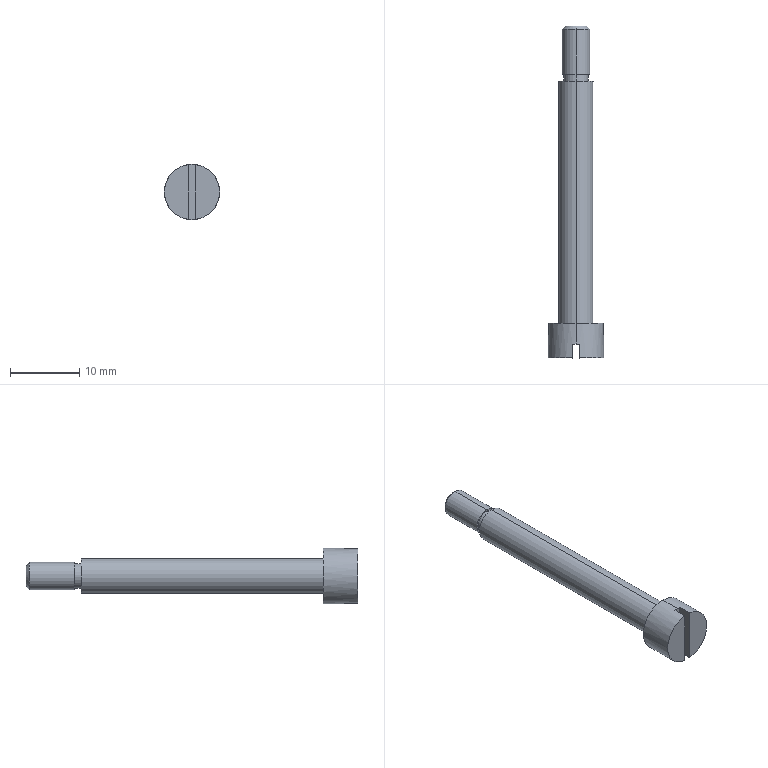Part | STEP file | 03-21 guide screw | 1 solid | 19 faces | box 8 x 48 x 8 mm | volume 1019 mm3 | plane 9 | cylinder 8 | cone 2 | commonest cylinder face diameters 3.5 x2 4 x2 5 x2 8 x2
STEP:
#1=CARTESIAN_POINT('',(0.,7.,1.5));
#2=VERTEX_POINT('',#1);
#3=CARTESIAN_POINT('',(0.,7.,-1.5));
#4=VERTEX_POINT('',#3);
#5=CARTESIAN_POINT('',(0.,7.,0.));
#6=DIRECTION('',(0.,1.,0.));
#7=DIRECTION('',(0.,0.,1.));
#8=AXIS2_PLACEMENT_3D('',#5,#6,#7);
#9=CIRCLE('',#8,1.5);
#10=EDGE_CURVE('',#2,#4,#9,.T.);
#11=ORIENTED_EDGE('',*,*,#10,.F.);
#12=CARTESIAN_POINT('',(0.,6.5,2.));
#13=VERTEX_POINT('',#12);
#14=CARTESIAN_POINT('',(0.,7.,1.5));
#15=DIRECTION('',(0.,-0.7071,0.7071));
#16=VECTOR('',#15,1000.);
#17=LINE('',#14,#16);
#18=EDGE_CURVE('',#2,#13,#17,.T.);
#19=ORIENTED_EDGE('',*,*,#18,.T.);
#20=CARTESIAN_POINT('',(0.,6.5,-2.));
#21=VERTEX_POINT('',#20);
#22=CARTESIAN_POINT('',(0.,6.5,0.));
#23=DIRECTION('',(0.,-1.,0.));
#24=DIRECTION('',(0.,0.,1.));
#25=AXIS2_PLACEMENT_3D('',#22,#23,#24);
#26=CIRCLE('',#25,2.);
#27=EDGE_CURVE('',#21,#13,#26,.T.);
#28=ORIENTED_EDGE('',*,*,#27,.F.);
#29=CARTESIAN_POINT('',(0.,7.,-1.5));
#30=DIRECTION('',(0.,-0.7071,-0.7071));
#31=VECTOR('',#30,1000.);
#32=LINE('',#29,#31);
#33=EDGE_CURVE('',#4,#21,#32,.T.);
#34=ORIENTED_EDGE('',*,*,#33,.F.);
#35=EDGE_LOOP('',(#11,#19,#28,#34));
#36=FACE_OUTER_BOUND('',#35,.T.);
#37=CARTESIAN_POINT('',(0.,7.,0.));
#38=DIRECTION('',(0.,-1.,0.));
#39=DIRECTION('',(0.,0.,-1.));
#40=AXIS2_PLACEMENT_3D('',#37,#38,#39);
#41=CONICAL_SURFACE('',#40,1.5,0.7854);
#42=ADVANCED_FACE('',(#36),#41,.T.);
#43=CARTESIAN_POINT('',(0.,-39.,-4.));
#44=VERTEX_POINT('',#43);
#45=CARTESIAN_POINT('',(0.5,-39.,-3.969));
#46=VERTEX_POINT('',#45);
#47=CARTESIAN_POINT('',(0.,-39.,0.));
#48=DIRECTION('',(0.,-1.,0.));
#49=DIRECTION('',(0.,0.,-1.));
#50=AXIS2_PLACEMENT_3D('',#47,#48,#49);
#51=CIRCLE('',#50,4.);
#52=EDGE_CURVE('',#44,#46,#51,.T.);
#53=ORIENTED_EDGE('',*,*,#52,.F.);
#54=CARTESIAN_POINT('',(0.,-36.,-4.));
#55=VERTEX_POINT('',#54);
#56=CARTESIAN_POINT('',(0.,-41.,-4.));
#57=DIRECTION('',(0.,1.,0.));
#58=VECTOR('',#57,1000.);
#59=LINE('',#56,#58);
#60=EDGE_CURVE('',#44,#55,#59,.T.);
#61=ORIENTED_EDGE('',*,*,#60,.T.);
#62=CARTESIAN_POINT('',(0.,-36.,4.));
#63=VERTEX_POINT('',#62);
#64=CARTESIAN_POINT('',(0.,-36.,0.));
#65=DIRECTION('',(0.,-1.,0.));
#66=DIRECTION('',(0.,0.,-1.));
#67=AXIS2_PLACEMENT_3D('',#64,#65,#66);
#68=CIRCLE('',#67,4.);
#69=EDGE_CURVE('',#55,#63,#68,.T.);
#70=ORIENTED_EDGE('',*,*,#69,.T.);
#71=CARTESIAN_POINT('',(0.,-39.,4.));
#72=VERTEX_POINT('',#71);
#73=CARTESIAN_POINT('',(0.,-41.,4.));
#74=DIRECTION('',(0.,1.,0.));
#75=VECTOR('',#74,1000.);
#76=LINE('',#73,#75);
#77=EDGE_CURVE('',#72,#63,#76,.T.);
#78=ORIENTED_EDGE('',*,*,#77,.F.);
#79=CARTESIAN_POINT('',(0.5,-39.,3.969));
#80=VERTEX_POINT('',#79);
#81=CARTESIAN_POINT('',(0.,-39.,0.));
#82=DIRECTION('',(0.,-1.,0.));
#83=DIRECTION('',(0.,0.,-1.));
#84=AXIS2_PLACEMENT_3D('',#81,#82,#83);
#85=CIRCLE('',#84,4.);
#86=EDGE_CURVE('',#80,#72,#85,.T.);
#87=ORIENTED_EDGE('',*,*,#86,.F.);
#88=CARTESIAN_POINT('',(0.5,-41.,3.969));
#89=VERTEX_POINT('',#88);
#90=CARTESIAN_POINT('',(0.5,-41.,3.969));
#91=DIRECTION('',(0.,-1.,0.));
#92=VECTOR('',#91,1000.);
#93=LINE('',#90,#92);
#94=EDGE_CURVE('',#80,#89,#93,.T.);
#95=ORIENTED_EDGE('',*,*,#94,.T.);
#96=CARTESIAN_POINT('',(0.5,-41.,-3.969));
#97=VERTEX_POINT('',#96);
#98=CARTESIAN_POINT('',(0.,-41.,0.));
#99=DIRECTION('',(0.,-1.,0.));
#100=DIRECTION('',(0.,0.,-1.));
#101=AXIS2_PLACEMENT_3D('',#98,#99,#100);
#102=CIRCLE('',#101,4.);
#103=EDGE_CURVE('',#97,#89,#102,.T.);
#104=ORIENTED_EDGE('',*,*,#103,.F.);
#105=CARTESIAN_POINT('',(0.5,-41.,-3.969));
#106=DIRECTION('',(0.,1.,0.));
#107=VECTOR('',#106,1000.);
#108=LINE('',#105,#107);
#109=EDGE_CURVE('',#97,#46,#108,.T.);
#110=ORIENTED_EDGE('',*,*,#109,.T.);
#111=EDGE_LOOP('',(#53,#61,#70,#78,#87,#95,#104,#110));
#112=FACE_OUTER_BOUND('',#111,.T.);
#113=CARTESIAN_POINT('',(0.,-41.,0.));
#114=DIRECTION('',(0.,1.,0.));
#115=DIRECTION('',(0.,0.,1.));
#116=AXIS2_PLACEMENT_3D('',#113,#114,#115);
#117=CYLINDRICAL_SURFACE('',#116,4.);
#118=ADVANCED_FACE('',(#112),#117,.T.);
#119=CARTESIAN_POINT('',(0.,-36.,-2.5));
#120=VERTEX_POINT('',#119);
#121=CARTESIAN_POINT('',(0.,-36.,2.5));
#122=VERTEX_POINT('',#121);
#123=CARTESIAN_POINT('',(0.,-36.,0.));
#124=DIRECTION('',(0.,-1.,0.));
#125=DIRECTION('',(0.,0.,-1.));
#126=AXIS2_PLACEMENT_3D('',#123,#124,#125);
#127=CIRCLE('',#126,2.5);
#128=EDGE_CURVE('',#120,#122,#127,.T.);
#129=ORIENTED_EDGE('',*,*,#128,.F.);
#130=CARTESIAN_POINT('',(0.,-1.,-2.5));
#131=VERTEX_POINT('',#130);
#132=CARTESIAN_POINT('',(0.,-36.,-2.5));
#133=DIRECTION('',(0.,1.,0.));
#134=VECTOR('',#133,1000.);
#135=LINE('',#132,#134);
#136=EDGE_CURVE('',#120,#131,#135,.T.);
#137=ORIENTED_EDGE('',*,*,#136,.T.);
#138=CARTESIAN_POINT('',(0.,-1.,2.5));
#139=VERTEX_POINT('',#138);
#140=CARTESIAN_POINT('',(0.,-1.,0.));
#141=DIRECTION('',(0.,-1.,0.));
#142=DIRECTION('',(0.,0.,-1.));
#143=AXIS2_PLACEMENT_3D('',#140,#141,#142);
#144=CIRCLE('',#143,2.5);
#145=EDGE_CURVE('',#131,#139,#144,.T.);
#146=ORIENTED_EDGE('',*,*,#145,.T.);
#147=CARTESIAN_POINT('',(0.,-36.,2.5));
#148=DIRECTION('',(0.,1.,0.));
#149=VECTOR('',#148,1000.);
#150=LINE('',#147,#149);
#151=EDGE_CURVE('',#122,#139,#150,.T.);
#152=ORIENTED_EDGE('',*,*,#151,.F.);
#153=EDGE_LOOP('',(#129,#137,#146,#152));
#154=FACE_OUTER_BOUND('',#153,.T.);
#155=CARTESIAN_POINT('',(0.,-36.,0.));
#156=DIRECTION('',(0.,1.,0.));
#157=DIRECTION('',(0.,0.,1.));
#158=AXIS2_PLACEMENT_3D('',#155,#156,#157);
#159=CYLINDRICAL_SURFACE('',#158,2.5);
#160=ADVANCED_FACE('',(#154),#159,.T.);
#161=CARTESIAN_POINT('',(0.,-1.,-1.75));
#162=VERTEX_POINT('',#161);
#163=CARTESIAN_POINT('',(0.,-1.,1.75));
#164=VERTEX_POINT('',#163);
#165=CARTESIAN_POINT('',(0.,-1.,0.));
#166=DIRECTION('',(0.,-1.,0.));
#167=DIRECTION('',(0.,0.,-1.));
#168=AXIS2_PLACEMENT_3D('',#165,#166,#167);
#169=CIRCLE('',#168,1.75);
#170=EDGE_CURVE('',#162,#164,#169,.T.);
#171=ORIENTED_EDGE('',*,*,#170,.F.);
#172=CARTESIAN_POINT('',(0.,0.,-1.75));
#173=VERTEX_POINT('',#172);
#174=CARTESIAN_POINT('',(0.,-1.,-1.75));
#175=DIRECTION('',(0.,1.,0.));
#176=VECTOR('',#175,1000.);
#177=LINE('',#174,#176);
#178=EDGE_CURVE('',#162,#173,#177,.T.);
#179=ORIENTED_EDGE('',*,*,#178,.T.);
#180=CARTESIAN_POINT('',(0.,0.,1.75));
#181=VERTEX_POINT('',#180);
#182=CARTESIAN_POINT('',(0.,0.,0.));
#183=DIRECTION('',(0.,-1.,0.));
#184=DIRECTION('',(0.,0.,1.));
#185=AXIS2_PLACEMENT_3D('',#182,#183,#184);
#186=CIRCLE('',#185,1.75);
#187=EDGE_CURVE('',#173,#181,#186,.T.);
#188=ORIENTED_EDGE('',*,*,#187,.T.);
#189=CARTESIAN_POINT('',(0.,-1.,1.75));
#190=DIRECTION('',(0.,1.,0.));
#191=VECTOR('',#190,1000.);
#192=LINE('',#189,#191);
#193=EDGE_CURVE('',#164,#181,#192,.T.);
#194=ORIENTED_EDGE('',*,*,#193,.F.);
#195=EDGE_LOOP('',(#171,#179,#188,#194));
#196=FACE_OUTER_BOUND('',#195,.T.);
#197=CARTESIAN_POINT('',(0.,-1.,0.));
#198=DIRECTION('',(0.,1.,0.));
#199=DIRECTION('',(0.,0.,1.));
#200=AXIS2_PLACEMENT_3D('',#197,#198,#199);
#201=CYLINDRICAL_SURFACE('',#200,1.75);
#202=ADVANCED_FACE('',(#196),#201,.T.);
#203=ORIENTED_EDGE('',*,*,#27,.T.);
#204=CARTESIAN_POINT('',(0.,0.,2.));
#205=VERTEX_POINT('',#204);
#206=CARTESIAN_POINT('',(0.,7.,2.));
#207=DIRECTION('',(0.,-1.,0.));
#208=VECTOR('',#207,1000.);
#209=LINE('',#206,#208);
#210=EDGE_CURVE('',#13,#205,#209,.T.);
#211=ORIENTED_EDGE('',*,*,#210,.T.);
#212=CARTESIAN_POINT('',(0.,0.,-2.));
#213=VERTEX_POINT('',#212);
#214=CARTESIAN_POINT('',(0.,0.,0.));
#215=DIRECTION('',(0.,1.,0.));
#216=DIRECTION('',(0.,0.,1.));
#217=AXIS2_PLACEMENT_3D('',#214,#215,#216);
#218=CIRCLE('',#217,2.);
#219=EDGE_CURVE('',#205,#213,#218,.T.);
#220=ORIENTED_EDGE('',*,*,#219,.T.);
#221=CARTESIAN_POINT('',(0.,7.,-2.));
#222=DIRECTION('',(0.,-1.,0.));
#223=VECTOR('',#222,1000.);
#224=LINE('',#221,#223);
#225=EDGE_CURVE('',#21,#213,#224,.T.);
#226=ORIENTED_EDGE('',*,*,#225,.F.);
#227=EDGE_LOOP('',(#203,#211,#220,#226));
#228=FACE_OUTER_BOUND('',#227,.T.);
#229=CARTESIAN_POINT('',(0.,7.,0.));
#230=DIRECTION('',(0.,-1.,0.));
#231=DIRECTION('',(0.,0.,-1.));
#232=AXIS2_PLACEMENT_3D('',#229,#230,#231);
#233=CYLINDRICAL_SURFACE('',#232,2.);
#234=ADVANCED_FACE('',(#228),#233,.T.);
#235=CARTESIAN_POINT('',(0.5,-41.,0.));
#236=DIRECTION('',(0.,0.,1.));
#237=VECTOR('',#236,1000.);
#238=LINE('',#235,#237);
#239=EDGE_CURVE('',#97,#89,#238,.T.);
#240=ORIENTED_EDGE('',*,*,#239,.F.);
#241=ORIENTED_EDGE('',*,*,#103,.T.);
#242=EDGE_LOOP('',(#240,#241));
#243=FACE_OUTER_BOUND('',#242,.T.);
#244=CARTESIAN_POINT('',(0.,-41.,0.));
#245=DIRECTION('',(0.,-1.,0.));
#246=DIRECTION('',(0.,0.,-1.));
#247=AXIS2_PLACEMENT_3D('',#244,#245,#246);
#248=PLANE('',#247);
#249=ADVANCED_FACE('',(#243),#248,.T.);
#250=CARTESIAN_POINT('',(0.,0.,0.));
#251=DIRECTION('',(0.,1.,0.));
#252=DIRECTION('',(0.,0.,1.));
#253=AXIS2_PLACEMENT_3D('',#250,#251,#252);
#254=CIRCLE('',#253,2.);
#255=EDGE_CURVE('',#213,#205,#254,.T.);
#256=ORIENTED_EDGE('',*,*,#255,.F.);
#257=ORIENTED_EDGE('',*,*,#219,.F.);
#258=EDGE_LOOP('',(#256,#257));
#259=FACE_OUTER_BOUND('',#258,.T.);
#260=CARTESIAN_POINT('',(0.,0.,0.));
#261=DIRECTION('',(0.,-1.,0.));
#262=DIRECTION('',(0.,0.,1.));
#263=AXIS2_PLACEMENT_3D('',#260,#261,#262);
#264=CIRCLE('',#263,1.75);
#265=EDGE_CURVE('',#181,#173,#264,.T.);
#266=ORIENTED_EDGE('',*,*,#265,.F.);
#267=ORIENTED_EDGE('',*,*,#187,.F.);
#268=EDGE_LOOP('',(#266,#267));
#269=FACE_BOUND('',#268,.T.);
#270=CARTESIAN_POINT('',(0.,0.,0.));
#271=DIRECTION('',(0.,1.,0.));
#272=DIRECTION('',(0.,0.,1.));
#273=AXIS2_PLACEMENT_3D('',#270,#271,#272);
#274=PLANE('',#273);
#275=ADVANCED_FACE('',(#259,#269),#274,.F.);
#276=ORIENTED_EDGE('',*,*,#210,.F.);
#277=CARTESIAN_POINT('',(0.,6.5,0.));
#278=DIRECTION('',(0.,-1.,0.));
#279=DIRECTION('',(0.,0.,1.));
#280=AXIS2_PLACEMENT_3D('',#277,#278,#279);
#281=CIRCLE('',#280,2.);
#282=EDGE_CURVE('',#13,#21,#281,.T.);
#283=ORIENTED_EDGE('',*,*,#282,.T.);
#284=ORIENTED_EDGE('',*,*,#225,.T.);
#285=ORIENTED_EDGE('',*,*,#255,.T.);
#286=EDGE_LOOP('',(#276,#283,#284,#285));
#287=FACE_OUTER_BOUND('',#286,.T.);
#288=CARTESIAN_POINT('',(0.,7.,0.));
#289=DIRECTION('',(0.,-1.,0.));
#290=DIRECTION('',(0.,0.,-1.));
#291=AXIS2_PLACEMENT_3D('',#288,#289,#290);
#292=CYLINDRICAL_SURFACE('',#291,2.);
#293=ADVANCED_FACE('',(#287),#292,.T.);
#294=CARTESIAN_POINT('',(0.,7.,0.));
#295=DIRECTION('',(0.,1.,0.));
#296=DIRECTION('',(0.,0.,1.));
#297=AXIS2_PLACEMENT_3D('',#294,#295,#296);
#298=CIRCLE('',#297,1.5);
#299=EDGE_CURVE('',#4,#2,#298,.T.);
#300=ORIENTED_EDGE('',*,*,#299,.T.);
#301=ORIENTED_EDGE('',*,*,#10,.T.);
#302=EDGE_LOOP('',(#300,#301));
#303=FACE_OUTER_BOUND('',#302,.T.);
#304=CARTESIAN_POINT('',(0.,7.,0.));
#305=DIRECTION('',(0.,1.,0.));
#306=DIRECTION('',(0.,0.,1.));
#307=AXIS2_PLACEMENT_3D('',#304,#305,#306);
#308=PLANE('',#307);
#309=ADVANCED_FACE('',(#303),#308,.T.);
#310=ORIENTED_EDGE('',*,*,#178,.F.);
#311=CARTESIAN_POINT('',(0.,-1.,0.));
#312=DIRECTION('',(0.,-1.,0.));
#313=DIRECTION('',(0.,0.,-1.));
#314=AXIS2_PLACEMENT_3D('',#311,#312,#313);
#315=CIRCLE('',#314,1.75);
#316=EDGE_CURVE('',#164,#162,#315,.T.);
#317=ORIENTED_EDGE('',*,*,#316,.F.);
#318=ORIENTED_EDGE('',*,*,#193,.T.);
#319=ORIENTED_EDGE('',*,*,#265,.T.);
#320=EDGE_LOOP('',(#310,#317,#318,#319));
#321=FACE_OUTER_BOUND('',#320,.T.);
#322=CARTESIAN_POINT('',(0.,-1.,0.));
#323=DIRECTION('',(0.,1.,0.));
#324=DIRECTION('',(0.,0.,1.));
#325=AXIS2_PLACEMENT_3D('',#322,#323,#324);
#326=CYLINDRICAL_SURFACE('',#325,1.75);
#327=ADVANCED_FACE('',(#321),#326,.T.);
#328=CARTESIAN_POINT('',(0.,-1.,0.));
#329=DIRECTION('',(0.,-1.,0.));
#330=DIRECTION('',(0.,0.,-1.));
#331=AXIS2_PLACEMENT_3D('',#328,#329,#330);
#332=CIRCLE('',#331,2.5);
#333=EDGE_CURVE('',#139,#131,#332,.T.);
#334=ORIENTED_EDGE('',*,*,#333,.F.);
#335=ORIENTED_EDGE('',*,*,#145,.F.);
#336=EDGE_LOOP('',(#334,#335));
#337=FACE_OUTER_BOUND('',#336,.T.);
#338=ORIENTED_EDGE('',*,*,#316,.T.);
#339=ORIENTED_EDGE('',*,*,#170,.T.);
#340=EDGE_LOOP('',(#338,#339));
#341=FACE_BOUND('',#340,.T.);
#342=CARTESIAN_POINT('',(0.,-1.,0.));
#343=DIRECTION('',(0.,-1.,0.));
#344=DIRECTION('',(0.,0.,-1.));
#345=AXIS2_PLACEMENT_3D('',#342,#343,#344);
#346=PLANE('',#345);
#347=ADVANCED_FACE('',(#337,#341),#346,.F.);
#348=ORIENTED_EDGE('',*,*,#136,.F.);
#349=CARTESIAN_POINT('',(0.,-36.,0.));
#350=DIRECTION('',(0.,-1.,0.));
#351=DIRECTION('',(0.,0.,-1.));
#352=AXIS2_PLACEMENT_3D('',#349,#350,#351);
#353=CIRCLE('',#352,2.5);
#354=EDGE_CURVE('',#122,#120,#353,.T.);
#355=ORIENTED_EDGE('',*,*,#354,.F.);
#356=ORIENTED_EDGE('',*,*,#151,.T.);
#357=ORIENTED_EDGE('',*,*,#333,.T.);
#358=EDGE_LOOP('',(#348,#355,#356,#357));
#359=FACE_OUTER_BOUND('',#358,.T.);
#360=CARTESIAN_POINT('',(0.,-36.,0.));
#361=DIRECTION('',(0.,1.,0.));
#362=DIRECTION('',(0.,0.,1.));
#363=AXIS2_PLACEMENT_3D('',#360,#361,#362);
#364=CYLINDRICAL_SURFACE('',#363,2.5);
#365=ADVANCED_FACE('',(#359),#364,.T.);
#366=CARTESIAN_POINT('',(0.,-36.,0.));
#367=DIRECTION('',(0.,-1.,0.));
#368=DIRECTION('',(0.,0.,-1.));
#369=AXIS2_PLACEMENT_3D('',#366,#367,#368);
#370=CIRCLE('',#369,4.);
#371=EDGE_CURVE('',#63,#55,#370,.T.);
#372=ORIENTED_EDGE('',*,*,#371,.F.);
#373=ORIENTED_EDGE('',*,*,#69,.F.);
#374=EDGE_LOOP('',(#372,#373));
#375=FACE_OUTER_BOUND('',#374,.T.);
#376=ORIENTED_EDGE('',*,*,#354,.T.);
#377=ORIENTED_EDGE('',*,*,#128,.T.);
#378=EDGE_LOOP('',(#376,#377));
#379=FACE_BOUND('',#378,.T.);
#380=CARTESIAN_POINT('',(0.,-36.,0.));
#381=DIRECTION('',(0.,-1.,0.));
#382=DIRECTION('',(0.,0.,-1.));
#383=AXIS2_PLACEMENT_3D('',#380,#381,#382);
#384=PLANE('',#383);
#385=ADVANCED_FACE('',(#375,#379),#384,.F.);
#386=ORIENTED_EDGE('',*,*,#60,.F.);
#387=CARTESIAN_POINT('',(-0.5,-39.,-3.969));
#388=VERTEX_POINT('',#387);
#389=CARTESIAN_POINT('',(0.,-39.,0.));
#390=DIRECTION('',(0.,-1.,0.));
#391=DIRECTION('',(0.,0.,-1.));
#392=AXIS2_PLACEMENT_3D('',#389,#390,#391);
#393=CIRCLE('',#392,4.);
#394=EDGE_CURVE('',#388,#44,#393,.T.);
#395=ORIENTED_EDGE('',*,*,#394,.F.);
#396=CARTESIAN_POINT('',(-0.5,-41.,-3.969));
#397=VERTEX_POINT('',#396);
#398=CARTESIAN_POINT('',(-0.5,-41.,-3.969));
#399=DIRECTION('',(0.,-1.,0.));
#400=VECTOR('',#399,1000.);
#401=LINE('',#398,#400);
#402=EDGE_CURVE('',#388,#397,#401,.T.);
#403=ORIENTED_EDGE('',*,*,#402,.T.);
#404=CARTESIAN_POINT('',(-0.5,-41.,3.969));
#405=VERTEX_POINT('',#404);
#406=CARTESIAN_POINT('',(0.,-41.,0.));
#407=DIRECTION('',(0.,-1.,0.));
#408=DIRECTION('',(0.,0.,-1.));
#409=AXIS2_PLACEMENT_3D('',#406,#407,#408);
#410=CIRCLE('',#409,4.);
#411=EDGE_CURVE('',#405,#397,#410,.T.);
#412=ORIENTED_EDGE('',*,*,#411,.F.);
#413=CARTESIAN_POINT('',(-0.5,-39.,3.969));
#414=VERTEX_POINT('',#413);
#415=CARTESIAN_POINT('',(-0.5,-41.,3.969));
#416=DIRECTION('',(0.,1.,0.));
#417=VECTOR('',#416,1000.);
#418=LINE('',#415,#417);
#419=EDGE_CURVE('',#405,#414,#418,.T.);
#420=ORIENTED_EDGE('',*,*,#419,.T.);
#421=CARTESIAN_POINT('',(0.,-39.,0.));
#422=DIRECTION('',(0.,-1.,0.));
#423=DIRECTION('',(0.,0.,-1.));
#424=AXIS2_PLACEMENT_3D('',#421,#422,#423);
#425=CIRCLE('',#424,4.);
#426=EDGE_CURVE('',#72,#414,#425,.T.);
#427=ORIENTED_EDGE('',*,*,#426,.F.);
#428=ORIENTED_EDGE('',*,*,#77,.T.);
#429=ORIENTED_EDGE('',*,*,#371,.T.);
#430=EDGE_LOOP('',(#386,#395,#403,#412,#420,#427,#428,#429));
#431=FACE_OUTER_BOUND('',#430,.T.);
#432=CARTESIAN_POINT('',(0.,-41.,0.));
#433=DIRECTION('',(0.,1.,0.));
#434=DIRECTION('',(0.,0.,1.));
#435=AXIS2_PLACEMENT_3D('',#432,#433,#434);
#436=CYLINDRICAL_SURFACE('',#435,4.);
#437=ADVANCED_FACE('',(#431),#436,.T.);
#438=CARTESIAN_POINT('',(-0.5,-41.,0.));
#439=DIRECTION('',(0.,0.,-1.));
#440=VECTOR('',#439,1000.);
#441=LINE('',#438,#440);
#442=EDGE_CURVE('',#405,#397,#441,.T.);
#443=ORIENTED_EDGE('',*,*,#442,.F.);
#444=ORIENTED_EDGE('',*,*,#411,.T.);
#445=EDGE_LOOP('',(#443,#444));
#446=FACE_OUTER_BOUND('',#445,.T.);
#447=CARTESIAN_POINT('',(0.,-41.,0.));
#448=DIRECTION('',(0.,-1.,0.));
#449=DIRECTION('',(0.,0.,-1.));
#450=AXIS2_PLACEMENT_3D('',#447,#448,#449);
#451=PLANE('',#450);
#452=ADVANCED_FACE('',(#446),#451,.T.);
#453=ORIENTED_EDGE('',*,*,#18,.F.);
#454=ORIENTED_EDGE('',*,*,#299,.F.);
#455=ORIENTED_EDGE('',*,*,#33,.T.);
#456=ORIENTED_EDGE('',*,*,#282,.F.);
#457=EDGE_LOOP('',(#453,#454,#455,#456));
#458=FACE_OUTER_BOUND('',#457,.T.);
#459=CARTESIAN_POINT('',(0.,7.,0.));
#460=DIRECTION('',(0.,-1.,0.));
#461=DIRECTION('',(0.,0.,-1.));
#462=AXIS2_PLACEMENT_3D('',#459,#460,#461);
#463=CONICAL_SURFACE('',#462,1.5,0.7854);
#464=ADVANCED_FACE('',(#458),#463,.T.);
#465=ORIENTED_EDGE('',*,*,#86,.T.);
#466=ORIENTED_EDGE('',*,*,#426,.T.);
#467=CARTESIAN_POINT('',(-0.5,-39.,4.171));
#468=DIRECTION('',(0.,0.,-1.));
#469=VECTOR('',#468,1000.);
#470=LINE('',#467,#469);
#471=EDGE_CURVE('',#414,#388,#470,.T.);
#472=ORIENTED_EDGE('',*,*,#471,.T.);
#473=ORIENTED_EDGE('',*,*,#394,.T.);
#474=ORIENTED_EDGE('',*,*,#52,.T.);
#475=CARTESIAN_POINT('',(0.5,-39.,4.171));
#476=DIRECTION('',(0.,0.,1.));
#477=VECTOR('',#476,1000.);
#478=LINE('',#475,#477);
#479=EDGE_CURVE('',#46,#80,#478,.T.);
#480=ORIENTED_EDGE('',*,*,#479,.T.);
#481=EDGE_LOOP('',(#465,#466,#472,#473,#474,#480));
#482=FACE_OUTER_BOUND('',#481,.T.);
#483=CARTESIAN_POINT('',(0.5,-39.,-4.171));
#484=DIRECTION('',(0.,-1.,0.));
#485=DIRECTION('',(0.,0.,-1.));
#486=AXIS2_PLACEMENT_3D('',#483,#484,#485);
#487=PLANE('',#486);
#488=ADVANCED_FACE('',(#482),#487,.T.);
#489=ORIENTED_EDGE('',*,*,#239,.T.);
#490=ORIENTED_EDGE('',*,*,#94,.F.);
#491=ORIENTED_EDGE('',*,*,#479,.F.);
#492=ORIENTED_EDGE('',*,*,#109,.F.);
#493=EDGE_LOOP('',(#489,#490,#491,#492));
#494=FACE_OUTER_BOUND('',#493,.T.);
#495=CARTESIAN_POINT('',(0.5,-39.,4.171));
#496=DIRECTION('',(1.,0.,0.));
#497=DIRECTION('',(0.,0.,-1.));
#498=AXIS2_PLACEMENT_3D('',#495,#496,#497);
#499=PLANE('',#498);
#500=ADVANCED_FACE('',(#494),#499,.F.);
#501=ORIENTED_EDGE('',*,*,#442,.T.);
#502=ORIENTED_EDGE('',*,*,#402,.F.);
#503=ORIENTED_EDGE('',*,*,#471,.F.);
#504=ORIENTED_EDGE('',*,*,#419,.F.);
#505=EDGE_LOOP('',(#501,#502,#503,#504));
#506=FACE_OUTER_BOUND('',#505,.T.);
#507=CARTESIAN_POINT('',(-0.5,-39.,4.171));
#508=DIRECTION('',(-1.,0.,0.));
#509=DIRECTION('',(0.,0.,1.));
#510=AXIS2_PLACEMENT_3D('',#507,#508,#509);
#511=PLANE('',#510);
#512=ADVANCED_FACE('',(#506),#511,.F.);
#513=CLOSED_SHELL('',(#42,#118,#160,#202,#234,#249,#275,#293,#309,#327,#347,#365,#385,#437,#452,#464,#488,#500,#512));
#514=MANIFOLD_SOLID_BREP('',#513);
#515=CARTESIAN_POINT('',(0.,0.,0.));
#516=DIRECTION('',(0.,0.,1.));
#517=DIRECTION('',(1.,0.,0.));
#518=AXIS2_PLACEMENT_3D('',#515,#516,#517);
#519=(LENGTH_UNIT()NAMED_UNIT(*)SI_UNIT(.MILLI.,.METRE.));
#520=UNCERTAINTY_MEASURE_WITH_UNIT(LENGTH_MEASURE(0.00001),#519,'','');
#521=(NAMED_UNIT(*)PLANE_ANGLE_UNIT()SI_UNIT($,.RADIAN.));
#522=(NAMED_UNIT(*)SI_UNIT($,.STERADIAN.)SOLID_ANGLE_UNIT());
#523=(GEOMETRIC_REPRESENTATION_CONTEXT(3)GLOBAL_UNCERTAINTY_ASSIGNED_CONTEXT((#520))GLOBAL_UNIT_ASSIGNED_CONTEXT((#519,#521,#522))REPRESENTATION_CONTEXT('',''));
#524=ADVANCED_BREP_SHAPE_REPRESENTATION('',(#514,#518),#523);